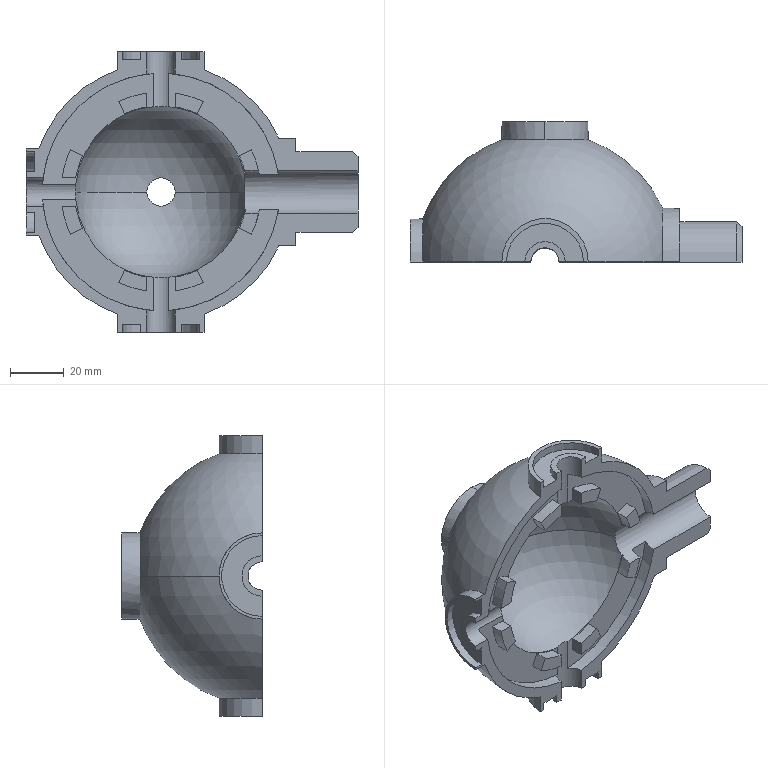Part | SolidWorks | features ICE 15, MirrorPattern 1, RevCut 1, Revolution 1, StudWizard 1 | 1 solid | 95 faces | box 123 x 52 x 104 mm | volume 156554 mm3 | plane 47 | cylinder 43 | sphere 4 | cone 1 | commonest cylinder face diameters 64 x9 74 x9 10.5 x5 32 x5 28.5 x4 88 x4